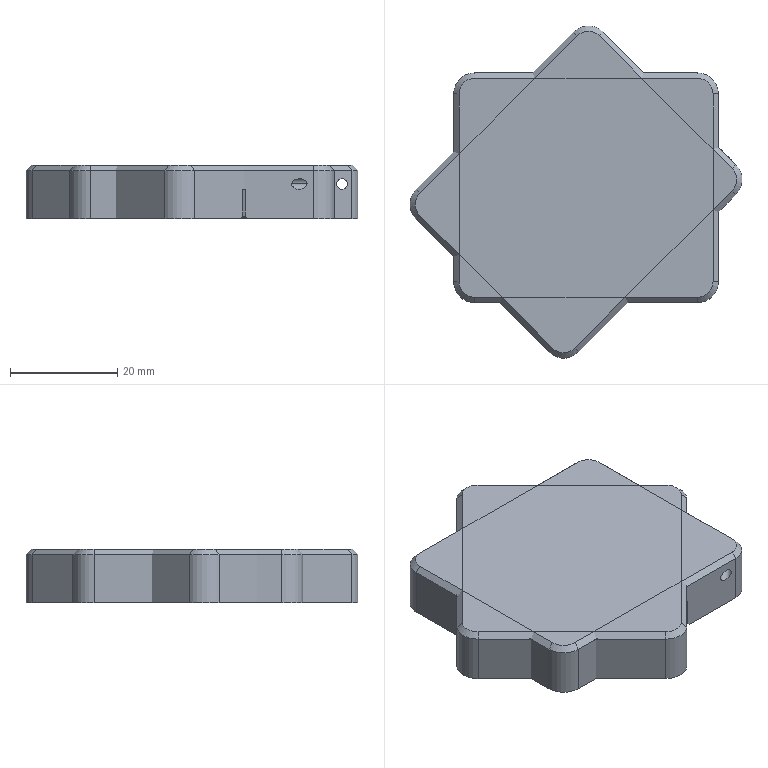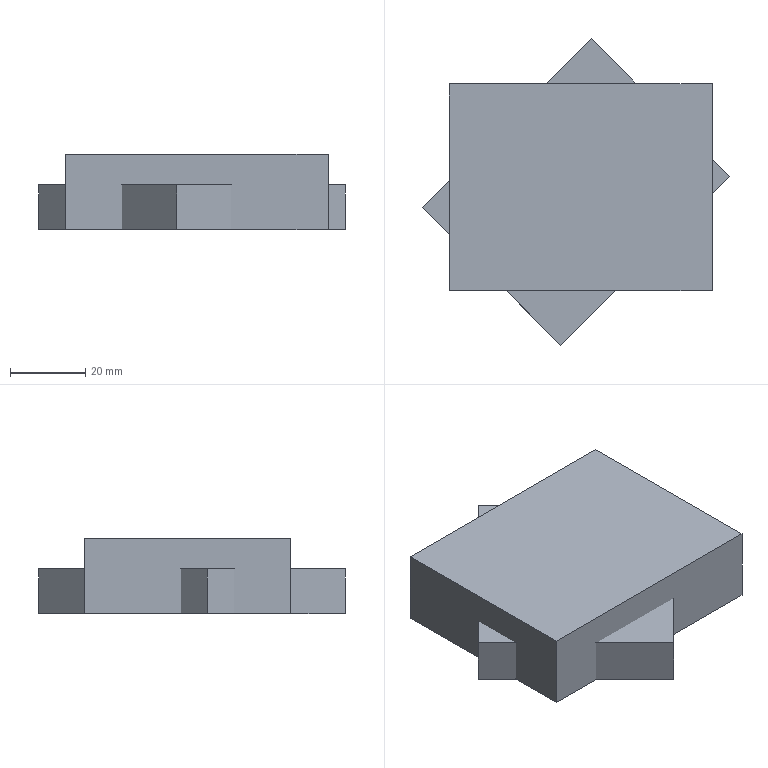CAM job | NX | 3+2 milling, drilling | part box 61.954 x 61.954 x 10 mm | stock box 81.605 x 81.605 x 20 mm
Tools:
number,name,description,diameter,corner_radius,flute_length,length,flutes
6,D2开粗,D2,2.0,0.0,6.0,50.0,2
3,D3精光,D3,3.0,0.0,9.0,50.0,2
13,D6精光,D6,6.0,0.0,16.0,60.0,2
2,D12开粗,D12,12.0,0.0,30.0,75.0,2
5,D8倒角刀,DJ8-32,8.0,0.0,4.0,60.0,2
1,D50面刀,Milling Tool-5 Parameters,63.0,0.0,50.0,75.0,2
7,D2钻头,Drilling Tool,2.0,0.0,35.0,50.0,2
Operations:
program,operation,operation_type,tool,method,geometry_group,spindle_rpm,surface_speed,feed_per_tooth,feed_cut,feed_plunge,cut_length_mm,path_length_mm,cut_time_min,machine_time_min
XX-CNC1,PLANAR_MILL_5,PlanarMilling,D50面刀,METHOD,MCS_1,3500.0,100.0,0.1178,800.0,100.0,193.616,247.616,0.242,0.2474
XX-CNC1,ADAPTIVE_MILLING,CavityMilling,D12开粗,METHOD,W1,5500.0,100.0,0.1178,2000.0,100.0,3638.111,3849.011,1.757,1.778
XX-CNC1,ADAPTIVE_MILLING_COPY,CavityMilling,D6精光,METHOD,W1,5500.0,100.0,0.1178,2000.0,100.0,39.304,190.683,0.0197,0.0348
XX-CNC1,PLANAR_MILL,PlanarMilling,D6精光,METHOD,W1,4500.0,100.0,0.1178,800.0,100.0,413.651,493.651,0.5171,0.5251
XX-CNC1,PLANAR_MILL_1,PlanarMilling,D6精光,METHOD,W1,4500.0,100.0,0.1178,800.0,100.0,315.601,380.601,0.3945,0.401
XX-CNC1,PLANAR_MILL_1_COPY,PlanarMilling,D6精光,METHOD,W1,4500.0,100.0,0.1178,800.0,100.0,127.035,192.036,0.1588,0.1653
XX-CNC1,PLANAR_MILL_2,PlanarMilling,D3精光,METHOD,W1,3500.0,100.0,0.1178,600.0,100.0,306.089,658.258,0.5101,0.5454
XX-CNC1,PLANAR_MILL_2_COPY,PlanarMilling,D3精光,METHOD,W1,3500.0,32.0,0.0286,200.0,100.0,72.057,427.529,0.3603,0.3958
XX-CNC1,PLANAR_MILL_3,PlanarMilling,D8倒角刀,METHOD,W1,3500.0,87.0,0.1143,800.0,100.0,131.889,188.889,0.1649,0.1706
XX-CNC1,PLANAR_MILL_3_COPY,PlanarMilling,D8倒角刀,METHOD,W1,3500.0,87.0,0.1143,800.0,100.0,187.118,244.118,0.2339,0.2396
XX-CNC1,PLANAR_MILL_3_COPY_COPY,PlanarMilling,D8倒角刀,METHOD,W1,3500.0,87.0,0.1143,800.0,100.0,51.415,397.914,0.0643,0.0989
XX-CNC2,ADAPTIVE_MILLING_1,CavityMilling,D12开粗,METHOD,W2,5500.0,207.0,0.2727,3000.0,100.0,4858.796,4912.596,1.62,1.625
XX-CNC2,一刀光面_COPY,VolumeBased25DMillingOperation,D50面刀,METHOD,MCS_2,3500.0,1187.0,0.1143,800.0,100.0,124.36,180.36,0.1554,0.161
XX-CNC2,PLANAR_MILL_3_COPY_COPY_COPY,PlanarMilling,D8倒角刀,METHOD,MCS_2,3500.0,87.0,0.1143,800.0,100.0,195.516,255.516,0.2444,0.2504
XX-CNC3,DRILLING,Operation,D2开粗,METHOD,MCS_3,3000.0,18.0,0.005,30.0,0.0,6.0,15.0,0.2,0.2009
XX-CNC3,DRILLING_COPY,Operation,D2钻头,METHOD,MCS_3,3000.0,18.0,0.005,30.0,0.0,16.0,35.0,0.5333,0.5352
XX-CNC5,PLANAR_MILL_4,PlanarMilling,D8倒角刀,METHOD,MCS_1,100.0,100.0,0.1178,1000.0,100.0,140.5,194.5,0.1405,0.1459